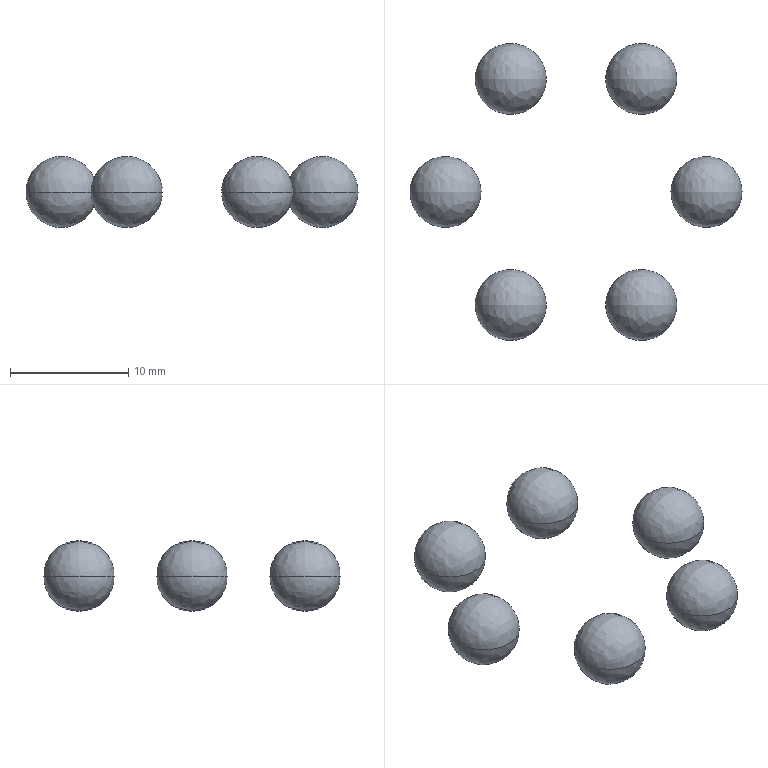Part | SolidWorks | 6 solids | 12 faces | box 28.05 x 25.096 x 5.88 mm | volume 678.568 mm3 | spline 12